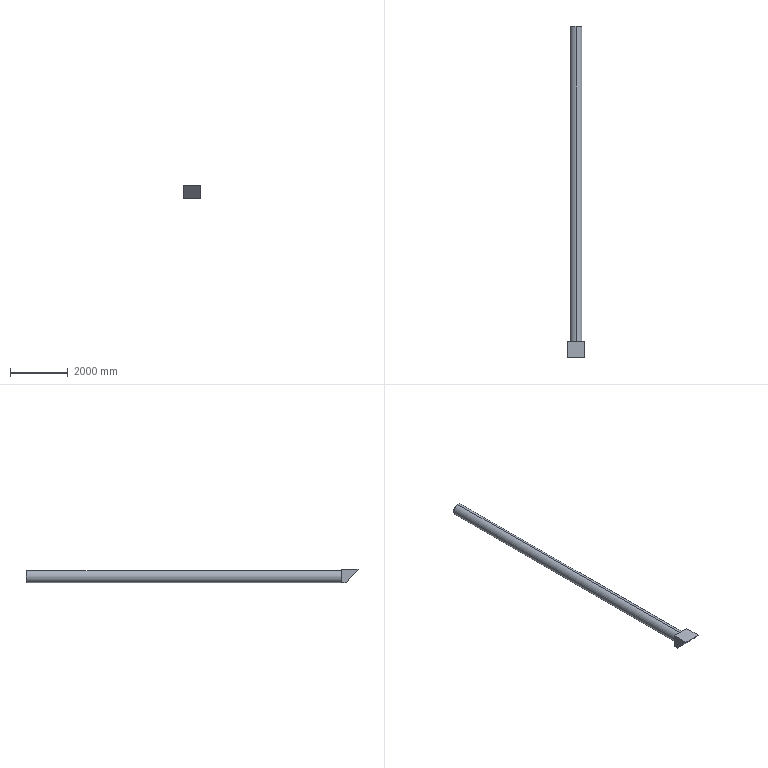Part | SolidWorks | features ICE 2, Chamfer 1, Extrusion 1 | 1 solid | 14 faces | box 600 x 11470 x 450 mm | volume 1002202960 mm3 | plane 8 | cylinder 4 | cone 2 | commonest cylinder face diameters 250 x2 410 x2
STEP:
#1=CARTESIAN_POINT('',(0.,10900.,175.));
#2=VERTEX_POINT('',#1);
#3=CARTESIAN_POINT('',(0.,10900.,-175.));
#4=VERTEX_POINT('',#3);
#5=CARTESIAN_POINT('',(0.,10900.,0.));
#6=DIRECTION('',(0.,1.,0.));
#7=DIRECTION('',(0.,0.,1.));
#8=AXIS2_PLACEMENT_3D('',#5,#6,#7);
#9=CIRCLE('',#8,175.);
#10=EDGE_CURVE('',#2,#4,#9,.T.);
#11=ORIENTED_EDGE('',*,*,#10,.F.);
#12=CARTESIAN_POINT('',(0.,10870.,205.));
#13=VERTEX_POINT('',#12);
#14=CARTESIAN_POINT('',(0.,10900.,175.));
#15=DIRECTION('',(0.,-0.7071,0.7071));
#16=VECTOR('',#15,1000.);
#17=LINE('',#14,#16);
#18=EDGE_CURVE('',#2,#13,#17,.T.);
#19=ORIENTED_EDGE('',*,*,#18,.T.);
#20=CARTESIAN_POINT('',(0.,10870.,-205.));
#21=VERTEX_POINT('',#20);
#22=CARTESIAN_POINT('',(0.,10870.,0.));
#23=DIRECTION('',(0.,-1.,0.));
#24=DIRECTION('',(0.,0.,1.));
#25=AXIS2_PLACEMENT_3D('',#22,#23,#24);
#26=CIRCLE('',#25,205.);
#27=EDGE_CURVE('',#21,#13,#26,.T.);
#28=ORIENTED_EDGE('',*,*,#27,.F.);
#29=CARTESIAN_POINT('',(0.,10900.,-175.));
#30=DIRECTION('',(0.,-0.7071,-0.7071));
#31=VECTOR('',#30,1000.);
#32=LINE('',#29,#31);
#33=EDGE_CURVE('',#4,#21,#32,.T.);
#34=ORIENTED_EDGE('',*,*,#33,.F.);
#35=EDGE_LOOP('',(#11,#19,#28,#34));
#36=FACE_OUTER_BOUND('',#35,.T.);
#37=CARTESIAN_POINT('',(0.,10900.,0.));
#38=DIRECTION('',(0.,-1.,0.));
#39=DIRECTION('',(0.,0.,-1.));
#40=AXIS2_PLACEMENT_3D('',#37,#38,#39);
#41=CONICAL_SURFACE('',#40,175.,0.7854);
#42=ADVANCED_FACE('',(#36),#41,.T.);
#43=CARTESIAN_POINT('',(0.,10900.,-125.));
#44=VERTEX_POINT('',#43);
#45=CARTESIAN_POINT('',(0.,10900.,125.));
#46=VERTEX_POINT('',#45);
#47=CARTESIAN_POINT('',(0.,10900.,0.));
#48=DIRECTION('',(0.,1.,0.));
#49=DIRECTION('',(0.,0.,1.));
#50=AXIS2_PLACEMENT_3D('',#47,#48,#49);
#51=CIRCLE('',#50,125.);
#52=EDGE_CURVE('',#44,#46,#51,.T.);
#53=ORIENTED_EDGE('',*,*,#52,.T.);
#54=CARTESIAN_POINT('',(0.,0.,125.));
#55=VERTEX_POINT('',#54);
#56=CARTESIAN_POINT('',(0.,10900.,125.));
#57=DIRECTION('',(0.,-1.,0.));
#58=VECTOR('',#57,1000.);
#59=LINE('',#56,#58);
#60=EDGE_CURVE('',#46,#55,#59,.T.);
#61=ORIENTED_EDGE('',*,*,#60,.T.);
#62=CARTESIAN_POINT('',(0.,0.,-125.));
#63=VERTEX_POINT('',#62);
#64=CARTESIAN_POINT('',(0.,0.,0.));
#65=DIRECTION('',(0.,1.,0.));
#66=DIRECTION('',(0.,0.,1.));
#67=AXIS2_PLACEMENT_3D('',#64,#65,#66);
#68=CIRCLE('',#67,125.);
#69=EDGE_CURVE('',#63,#55,#68,.T.);
#70=ORIENTED_EDGE('',*,*,#69,.F.);
#71=CARTESIAN_POINT('',(0.,10900.,-125.));
#72=DIRECTION('',(0.,-1.,0.));
#73=VECTOR('',#72,1000.);
#74=LINE('',#71,#73);
#75=EDGE_CURVE('',#44,#63,#74,.T.);
#76=ORIENTED_EDGE('',*,*,#75,.F.);
#77=EDGE_LOOP('',(#53,#61,#70,#76));
#78=FACE_OUTER_BOUND('',#77,.T.);
#79=CARTESIAN_POINT('',(0.,10900.,0.));
#80=DIRECTION('',(0.,-1.,0.));
#81=DIRECTION('',(0.,0.,-1.));
#82=AXIS2_PLACEMENT_3D('',#79,#80,#81);
#83=CYLINDRICAL_SURFACE('',#82,125.);
#84=ADVANCED_FACE('',(#78),#83,.F.);
#85=ORIENTED_EDGE('',*,*,#27,.T.);
#86=CARTESIAN_POINT('',(0.,-2.,205.));
#87=VERTEX_POINT('',#86);
#88=CARTESIAN_POINT('',(0.,10900.,205.));
#89=DIRECTION('',(0.,-1.,0.));
#90=VECTOR('',#89,1000.);
#91=LINE('',#88,#90);
#92=EDGE_CURVE('',#13,#87,#91,.T.);
#93=ORIENTED_EDGE('',*,*,#92,.T.);
#94=CARTESIAN_POINT('',(0.,-2.,-205.));
#95=VERTEX_POINT('',#94);
#96=CARTESIAN_POINT('',(0.,-2.,0.));
#97=DIRECTION('',(0.,-1.,0.));
#98=DIRECTION('',(0.,0.,-1.));
#99=AXIS2_PLACEMENT_3D('',#96,#97,#98);
#100=CIRCLE('',#99,205.);
#101=EDGE_CURVE('',#95,#87,#100,.T.);
#102=ORIENTED_EDGE('',*,*,#101,.F.);
#103=CARTESIAN_POINT('',(0.,10900.,-205.));
#104=DIRECTION('',(0.,-1.,0.));
#105=VECTOR('',#104,1000.);
#106=LINE('',#103,#105);
#107=EDGE_CURVE('',#21,#95,#106,.T.);
#108=ORIENTED_EDGE('',*,*,#107,.F.);
#109=EDGE_LOOP('',(#85,#93,#102,#108));
#110=FACE_OUTER_BOUND('',#109,.T.);
#111=CARTESIAN_POINT('',(0.,10900.,0.));
#112=DIRECTION('',(0.,-1.,0.));
#113=DIRECTION('',(0.,0.,-1.));
#114=AXIS2_PLACEMENT_3D('',#111,#112,#113);
#115=CYLINDRICAL_SURFACE('',#114,205.);
#116=ADVANCED_FACE('',(#110),#115,.T.);
#117=CARTESIAN_POINT('',(0.,10900.,0.));
#118=DIRECTION('',(0.,1.,0.));
#119=DIRECTION('',(0.,0.,1.));
#120=AXIS2_PLACEMENT_3D('',#117,#118,#119);
#121=CIRCLE('',#120,175.);
#122=EDGE_CURVE('',#4,#2,#121,.T.);
#123=ORIENTED_EDGE('',*,*,#122,.T.);
#124=ORIENTED_EDGE('',*,*,#10,.T.);
#125=EDGE_LOOP('',(#123,#124));
#126=FACE_OUTER_BOUND('',#125,.T.);
#127=ORIENTED_EDGE('',*,*,#52,.F.);
#128=CARTESIAN_POINT('',(0.,10900.,0.));
#129=DIRECTION('',(0.,1.,0.));
#130=DIRECTION('',(0.,0.,1.));
#131=AXIS2_PLACEMENT_3D('',#128,#129,#130);
#132=CIRCLE('',#131,125.);
#133=EDGE_CURVE('',#46,#44,#132,.T.);
#134=ORIENTED_EDGE('',*,*,#133,.F.);
#135=EDGE_LOOP('',(#127,#134));
#136=FACE_BOUND('',#135,.T.);
#137=CARTESIAN_POINT('',(0.,10900.,0.));
#138=DIRECTION('',(0.,1.,0.));
#139=DIRECTION('',(0.,0.,1.));
#140=AXIS2_PLACEMENT_3D('',#137,#138,#139);
#141=PLANE('',#140);
#142=ADVANCED_FACE('',(#126,#136),#141,.T.);
#143=ORIENTED_EDGE('',*,*,#92,.F.);
#144=CARTESIAN_POINT('',(0.,10870.,0.));
#145=DIRECTION('',(0.,-1.,0.));
#146=DIRECTION('',(0.,0.,1.));
#147=AXIS2_PLACEMENT_3D('',#144,#145,#146);
#148=CIRCLE('',#147,205.);
#149=EDGE_CURVE('',#13,#21,#148,.T.);
#150=ORIENTED_EDGE('',*,*,#149,.T.);
#151=ORIENTED_EDGE('',*,*,#107,.T.);
#152=CARTESIAN_POINT('',(0.,-2.,0.));
#153=DIRECTION('',(0.,-1.,0.));
#154=DIRECTION('',(0.,0.,-1.));
#155=AXIS2_PLACEMENT_3D('',#152,#153,#154);
#156=CIRCLE('',#155,205.);
#157=EDGE_CURVE('',#87,#95,#156,.T.);
#158=ORIENTED_EDGE('',*,*,#157,.F.);
#159=EDGE_LOOP('',(#143,#150,#151,#158));
#160=FACE_OUTER_BOUND('',#159,.T.);
#161=CARTESIAN_POINT('',(0.,10900.,0.));
#162=DIRECTION('',(0.,-1.,0.));
#163=DIRECTION('',(0.,0.,-1.));
#164=AXIS2_PLACEMENT_3D('',#161,#162,#163);
#165=CYLINDRICAL_SURFACE('',#164,205.);
#166=ADVANCED_FACE('',(#160),#165,.T.);
#167=ORIENTED_EDGE('',*,*,#60,.F.);
#168=ORIENTED_EDGE('',*,*,#133,.T.);
#169=ORIENTED_EDGE('',*,*,#75,.T.);
#170=CARTESIAN_POINT('',(0.,0.,0.));
#171=DIRECTION('',(0.,1.,0.));
#172=DIRECTION('',(0.,0.,1.));
#173=AXIS2_PLACEMENT_3D('',#170,#171,#172);
#174=CIRCLE('',#173,125.);
#175=EDGE_CURVE('',#55,#63,#174,.T.);
#176=ORIENTED_EDGE('',*,*,#175,.F.);
#177=EDGE_LOOP('',(#167,#168,#169,#176));
#178=FACE_OUTER_BOUND('',#177,.T.);
#179=CARTESIAN_POINT('',(0.,10900.,0.));
#180=DIRECTION('',(0.,-1.,0.));
#181=DIRECTION('',(0.,0.,-1.));
#182=AXIS2_PLACEMENT_3D('',#179,#180,#181);
#183=CYLINDRICAL_SURFACE('',#182,125.);
#184=ADVANCED_FACE('',(#178),#183,.F.);
#185=ORIENTED_EDGE('',*,*,#69,.T.);
#186=ORIENTED_EDGE('',*,*,#175,.T.);
#187=EDGE_LOOP('',(#185,#186));
#188=FACE_OUTER_BOUND('',#187,.T.);
#189=CARTESIAN_POINT('',(0.,0.,0.));
#190=DIRECTION('',(0.,-1.,0.));
#191=DIRECTION('',(0.,0.,-1.));
#192=AXIS2_PLACEMENT_3D('',#189,#190,#191);
#193=PLANE('',#192);
#194=ADVANCED_FACE('',(#188),#193,.F.);
#195=ORIENTED_EDGE('',*,*,#18,.F.);
#196=ORIENTED_EDGE('',*,*,#122,.F.);
#197=ORIENTED_EDGE('',*,*,#33,.T.);
#198=ORIENTED_EDGE('',*,*,#149,.F.);
#199=EDGE_LOOP('',(#195,#196,#197,#198));
#200=FACE_OUTER_BOUND('',#199,.T.);
#201=CARTESIAN_POINT('',(0.,10900.,0.));
#202=DIRECTION('',(0.,-1.,0.));
#203=DIRECTION('',(0.,0.,-1.));
#204=AXIS2_PLACEMENT_3D('',#201,#202,#203);
#205=CONICAL_SURFACE('',#204,175.,0.7854);
#206=ADVANCED_FACE('',(#200),#205,.T.);
#207=CARTESIAN_POINT('',(300.,-2.,-205.));
#208=VERTEX_POINT('',#207);
#209=CARTESIAN_POINT('',(-300.,-2.,-205.));
#210=DIRECTION('',(1.,0.,0.));
#211=VECTOR('',#210,1000.);
#212=LINE('',#209,#211);
#213=EDGE_CURVE('',#95,#208,#212,.T.);
#214=ORIENTED_EDGE('',*,*,#213,.F.);
#215=ORIENTED_EDGE('',*,*,#101,.T.);
#216=ORIENTED_EDGE('',*,*,#157,.T.);
#217=CARTESIAN_POINT('',(-300.,-2.,-205.));
#218=VERTEX_POINT('',#217);
#219=CARTESIAN_POINT('',(-300.,-2.,-205.));
#220=DIRECTION('',(1.,0.,0.));
#221=VECTOR('',#220,1000.);
#222=LINE('',#219,#221);
#223=EDGE_CURVE('',#218,#95,#222,.T.);
#224=ORIENTED_EDGE('',*,*,#223,.F.);
#225=CARTESIAN_POINT('',(-300.,-2.,245.));
#226=VERTEX_POINT('',#225);
#227=CARTESIAN_POINT('',(-300.,-2.,245.));
#228=DIRECTION('',(0.,0.,1.));
#229=VECTOR('',#228,1000.);
#230=LINE('',#227,#229);
#231=EDGE_CURVE('',#218,#226,#230,.T.);
#232=ORIENTED_EDGE('',*,*,#231,.T.);
#233=CARTESIAN_POINT('',(300.,-2.,245.));
#234=VERTEX_POINT('',#233);
#235=CARTESIAN_POINT('',(-300.,-2.,245.));
#236=DIRECTION('',(1.,0.,0.));
#237=VECTOR('',#236,1000.);
#238=LINE('',#235,#237);
#239=EDGE_CURVE('',#226,#234,#238,.T.);
#240=ORIENTED_EDGE('',*,*,#239,.T.);
#241=CARTESIAN_POINT('',(300.,-2.,245.));
#242=DIRECTION('',(0.,0.,1.));
#243=VECTOR('',#242,1000.);
#244=LINE('',#241,#243);
#245=EDGE_CURVE('',#208,#234,#244,.T.);
#246=ORIENTED_EDGE('',*,*,#245,.F.);
#247=EDGE_LOOP('',(#214,#215,#216,#224,#232,#240,#246));
#248=FACE_OUTER_BOUND('',#247,.T.);
#249=CARTESIAN_POINT('',(-300.,-2.,245.));
#250=DIRECTION('',(0.,1.,0.));
#251=DIRECTION('',(0.,0.,1.));
#252=AXIS2_PLACEMENT_3D('',#249,#250,#251);
#253=PLANE('',#252);
#254=ADVANCED_FACE('',(#248),#253,.T.);
#255=ORIENTED_EDGE('',*,*,#223,.T.);
#256=ORIENTED_EDGE('',*,*,#213,.T.);
#257=CARTESIAN_POINT('',(300.,-163.464,-205.));
#258=VERTEX_POINT('',#257);
#259=CARTESIAN_POINT('',(300.,-2.,-205.));
#260=DIRECTION('',(0.,1.,0.));
#261=VECTOR('',#260,1000.);
#262=LINE('',#259,#261);
#263=EDGE_CURVE('',#258,#208,#262,.T.);
#264=ORIENTED_EDGE('',*,*,#263,.F.);
#265=CARTESIAN_POINT('',(-300.,-163.464,-205.));
#266=VERTEX_POINT('',#265);
#267=CARTESIAN_POINT('',(-300.,-163.464,-205.));
#268=DIRECTION('',(1.,0.,0.));
#269=VECTOR('',#268,1000.);
#270=LINE('',#267,#269);
#271=EDGE_CURVE('',#266,#258,#270,.T.);
#272=ORIENTED_EDGE('',*,*,#271,.F.);
#273=CARTESIAN_POINT('',(-300.,-2.,-205.));
#274=DIRECTION('',(0.,1.,0.));
#275=VECTOR('',#274,1000.);
#276=LINE('',#273,#275);
#277=EDGE_CURVE('',#266,#218,#276,.T.);
#278=ORIENTED_EDGE('',*,*,#277,.T.);
#279=EDGE_LOOP('',(#255,#256,#264,#272,#278));
#280=FACE_OUTER_BOUND('',#279,.T.);
#281=CARTESIAN_POINT('',(-300.,-2.,-205.));
#282=DIRECTION('',(0.,0.,-1.));
#283=DIRECTION('',(0.,1.,0.));
#284=AXIS2_PLACEMENT_3D('',#281,#282,#283);
#285=PLANE('',#284);
#286=ADVANCED_FACE('',(#280),#285,.T.);
#287=ORIENTED_EDGE('',*,*,#271,.T.);
#288=CARTESIAN_POINT('',(300.,-569.911,245.));
#289=VERTEX_POINT('',#288);
#290=CARTESIAN_POINT('',(300.,-163.464,-205.));
#291=DIRECTION('',(0.,0.6703,-0.7421));
#292=VECTOR('',#291,1000.);
#293=LINE('',#290,#292);
#294=EDGE_CURVE('',#289,#258,#293,.T.);
#295=ORIENTED_EDGE('',*,*,#294,.F.);
#296=CARTESIAN_POINT('',(-300.,-569.911,245.));
#297=VERTEX_POINT('',#296);
#298=CARTESIAN_POINT('',(-300.,-569.911,245.));
#299=DIRECTION('',(1.,0.,0.));
#300=VECTOR('',#299,1000.);
#301=LINE('',#298,#300);
#302=EDGE_CURVE('',#297,#289,#301,.T.);
#303=ORIENTED_EDGE('',*,*,#302,.F.);
#304=CARTESIAN_POINT('',(-300.,-163.464,-205.));
#305=DIRECTION('',(0.,0.6703,-0.7421));
#306=VECTOR('',#305,1000.);
#307=LINE('',#304,#306);
#308=EDGE_CURVE('',#297,#266,#307,.T.);
#309=ORIENTED_EDGE('',*,*,#308,.T.);
#310=EDGE_LOOP('',(#287,#295,#303,#309));
#311=FACE_OUTER_BOUND('',#310,.T.);
#312=CARTESIAN_POINT('',(-300.,-163.464,-205.));
#313=DIRECTION('',(0.,-0.7421,-0.6703));
#314=DIRECTION('',(0.,0.6703,-0.7421));
#315=AXIS2_PLACEMENT_3D('',#312,#313,#314);
#316=PLANE('',#315);
#317=ADVANCED_FACE('',(#311),#316,.T.);
#318=ORIENTED_EDGE('',*,*,#302,.T.);
#319=CARTESIAN_POINT('',(300.,-569.911,245.));
#320=DIRECTION('',(0.,-1.,0.));
#321=VECTOR('',#320,1000.);
#322=LINE('',#319,#321);
#323=EDGE_CURVE('',#234,#289,#322,.T.);
#324=ORIENTED_EDGE('',*,*,#323,.F.);
#325=ORIENTED_EDGE('',*,*,#239,.F.);
#326=CARTESIAN_POINT('',(-300.,-569.911,245.));
#327=DIRECTION('',(0.,-1.,0.));
#328=VECTOR('',#327,1000.);
#329=LINE('',#326,#328);
#330=EDGE_CURVE('',#226,#297,#329,.T.);
#331=ORIENTED_EDGE('',*,*,#330,.T.);
#332=EDGE_LOOP('',(#318,#324,#325,#331));
#333=FACE_OUTER_BOUND('',#332,.T.);
#334=CARTESIAN_POINT('',(-300.,-569.911,245.));
#335=DIRECTION('',(0.,0.,1.));
#336=DIRECTION('',(1.,0.,0.));
#337=AXIS2_PLACEMENT_3D('',#334,#335,#336);
#338=PLANE('',#337);
#339=ADVANCED_FACE('',(#333),#338,.T.);
#340=ORIENTED_EDGE('',*,*,#231,.F.);
#341=ORIENTED_EDGE('',*,*,#277,.F.);
#342=ORIENTED_EDGE('',*,*,#308,.F.);
#343=ORIENTED_EDGE('',*,*,#330,.F.);
#344=EDGE_LOOP('',(#340,#341,#342,#343));
#345=FACE_OUTER_BOUND('',#344,.T.);
#346=CARTESIAN_POINT('',(-300.,0.,0.));
#347=DIRECTION('',(-1.,0.,0.));
#348=DIRECTION('',(0.,0.,1.));
#349=AXIS2_PLACEMENT_3D('',#346,#347,#348);
#350=PLANE('',#349);
#351=ADVANCED_FACE('',(#345),#350,.T.);
#352=ORIENTED_EDGE('',*,*,#245,.T.);
#353=ORIENTED_EDGE('',*,*,#323,.T.);
#354=ORIENTED_EDGE('',*,*,#294,.T.);
#355=ORIENTED_EDGE('',*,*,#263,.T.);
#356=EDGE_LOOP('',(#352,#353,#354,#355));
#357=FACE_OUTER_BOUND('',#356,.T.);
#358=CARTESIAN_POINT('',(300.,0.,0.));
#359=DIRECTION('',(-1.,0.,0.));
#360=DIRECTION('',(0.,0.,1.));
#361=AXIS2_PLACEMENT_3D('',#358,#359,#360);
#362=PLANE('',#361);
#363=ADVANCED_FACE('',(#357),#362,.F.);
#364=CLOSED_SHELL('',(#42,#84,#116,#142,#166,#184,#194,#206,#254,#286,#317,#339,#351,#363));
#365=MANIFOLD_SOLID_BREP('',#364);
#366=CARTESIAN_POINT('',(0.,0.,0.));
#367=DIRECTION('',(0.,0.,1.));
#368=DIRECTION('',(1.,0.,0.));
#369=AXIS2_PLACEMENT_3D('',#366,#367,#368);
#370=(LENGTH_UNIT()NAMED_UNIT(*)SI_UNIT(.MILLI.,.METRE.));
#371=UNCERTAINTY_MEASURE_WITH_UNIT(LENGTH_MEASURE(0.00001),#370,'','');
#372=(NAMED_UNIT(*)PLANE_ANGLE_UNIT()SI_UNIT($,.RADIAN.));
#373=(NAMED_UNIT(*)SI_UNIT($,.STERADIAN.)SOLID_ANGLE_UNIT());
#374=(GEOMETRIC_REPRESENTATION_CONTEXT(3)GLOBAL_UNCERTAINTY_ASSIGNED_CONTEXT((#371))GLOBAL_UNIT_ASSIGNED_CONTEXT((#370,#372,#373))REPRESENTATION_CONTEXT('',''));
#375=ADVANCED_BREP_SHAPE_REPRESENTATION('',(#365,#369),#374);